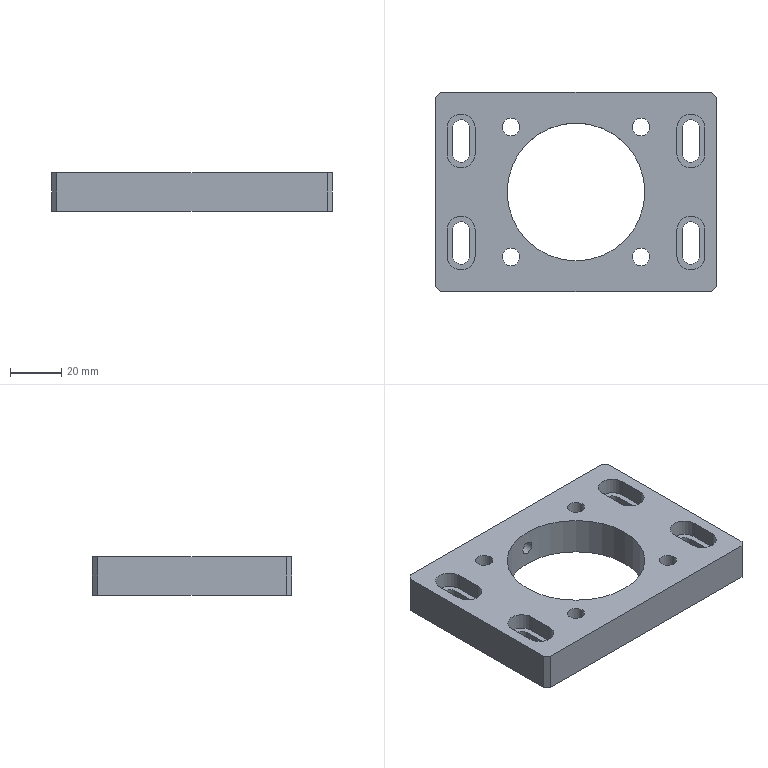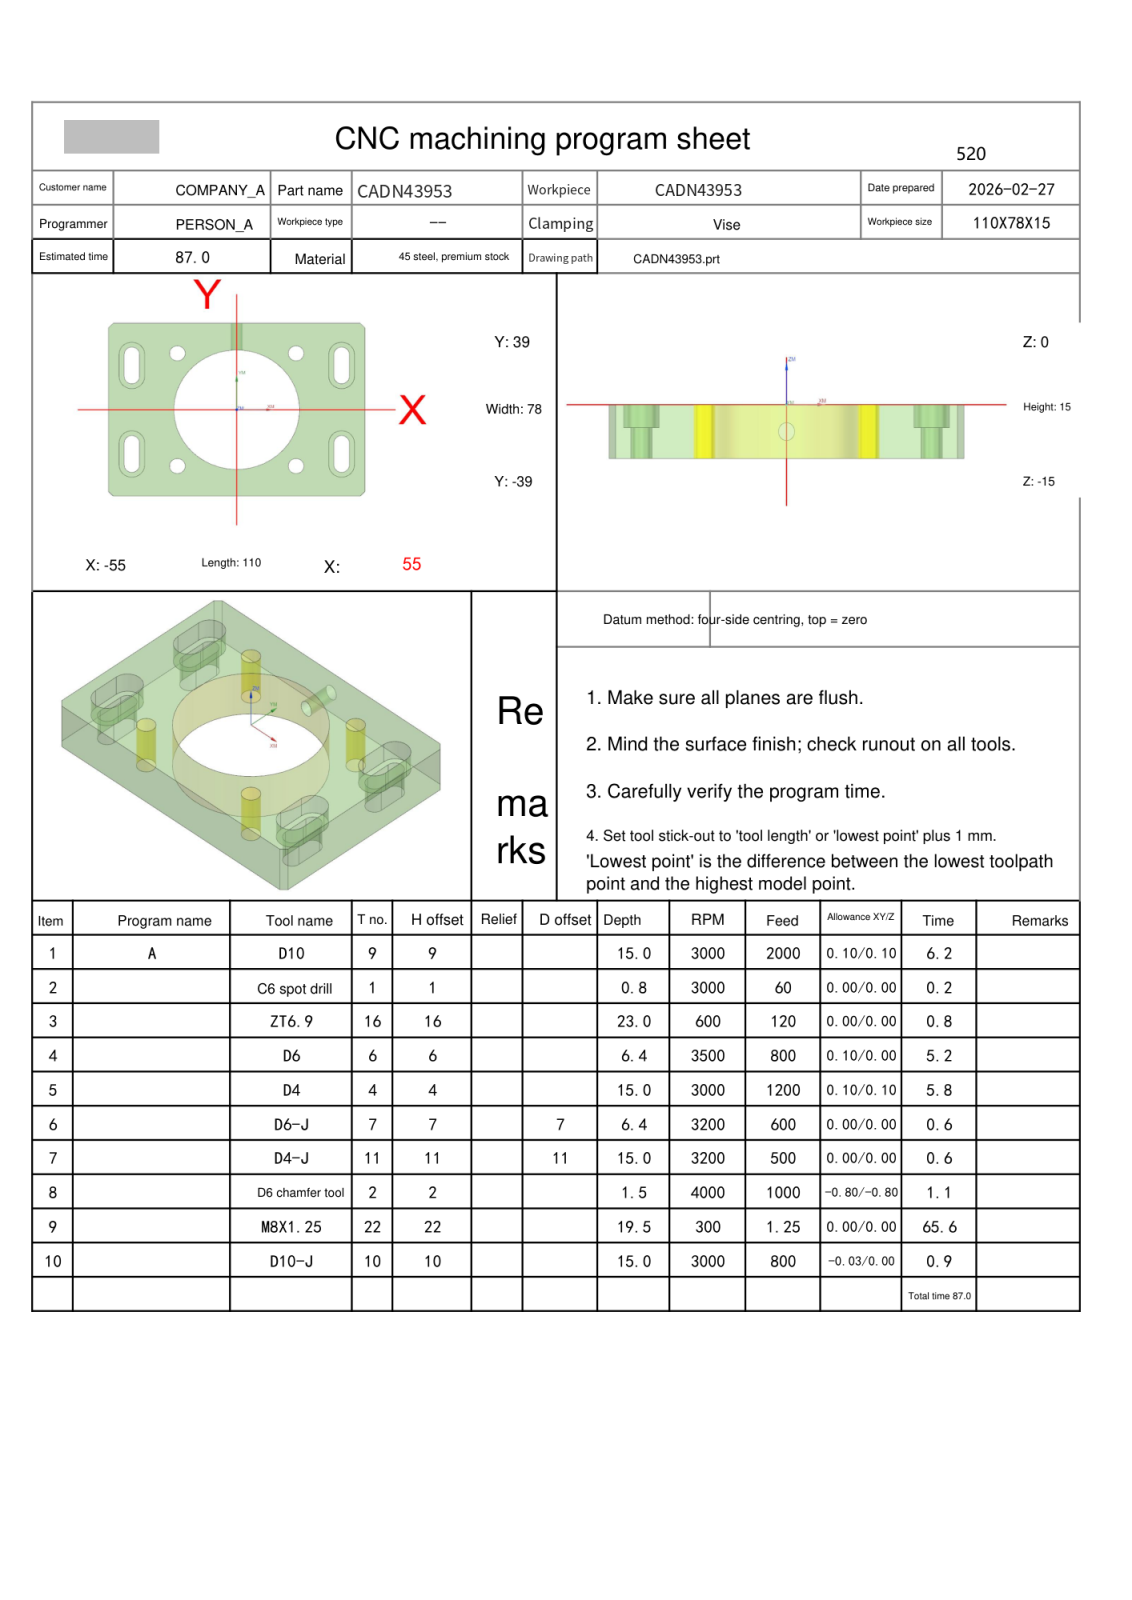NC program | NX | posted by the shop | part box 110 x 78 x 15 mm
Lines 4089 to 4469 of 4469:
N8 T02 M06
(D6 chamfer tool  D=6. R=0. H=02 ce=-0.80 di=0.00)
G00 G90 G54 X-26.256 Y26.956 M03 S4000
G43 H02 Z50.
M08
Z-1.
G01 Z-1.5 F500.
X-26.656
G03 X-28.156 Y25.456 I0.0 J-1.5
X-25.456 Y22.756 I2.7 J0.0
X-22.756 Y25.456 I0.0 J2.7
X-25.456 Y28.156 I-2.7 J0.0
X-28.156 Y25.456 I0.0 J-2.7
X-26.656 Y23.956 I1.5 J0.0
G01 X-26.256
Z-1.
G00 Z50.
X24.656 Y26.956
Z-1.
G01 Z-1.5
X24.256
G03 X22.756 Y25.456 I0.0 J-1.5
X25.456 Y22.756 I2.7 J0.0
X28.156 Y25.456 I0.0 J2.7
X25.456 Y28.156 I-2.7 J0.0
X22.756 Y25.456 I0.0 J-2.7
X24.256 Y23.956 I1.5 J0.0
G01 X24.656
Z-1.
G00 Z50.
Y-23.956
Z-1.
G01 Z-1.5
X24.256
G03 X22.756 Y-25.456 I0.0 J-1.5
X25.456 Y-28.156 I2.7 J0.0
X28.156 Y-25.456 I0.0 J2.7
X25.456 Y-22.756 I-2.7 J0.0
X22.756 Y-25.456 I0.0 J-2.7
X24.256 Y-26.956 I1.5 J0.0
G01 X24.656
Z-1.
G00 Z50.
X-26.256 Y-23.956
Z-1.
G01 Z-1.5
X-26.656
G03 X-28.156 Y-25.456 I0.0 J-1.5
X-25.456 Y-28.156 I2.7 J0.0
X-22.756 Y-25.456 I0.0 J2.7
X-25.456 Y-22.756 I-2.7 J0.0
X-28.156 Y-25.456 I0.0 J-2.7
X-26.656 Y-26.956 I1.5 J0.0
G01 X-26.256
Z-1.
G00 Z50.
G00 G90 X-.386 Y40.227 M03 S3500
Z50.
Z.172
G01 Z-1.2 F1000.
G03 X-.1 Y40.027 I1.286 J1.532
G01 X-.054 Y39.997
X0.0 Y40.
X53.
X53.259 Y39.966
X53.5 Y39.866
X53.707 Y39.707
X55.707 Y37.707
X55.866 Y37.5
X55.966 Y37.259
X56. Y37.
Y-37.
X55.966 Y-37.259
X55.866 Y-37.5
X55.707 Y-37.707
X53.707 Y-39.707
X53.5 Y-39.866
X53.259 Y-39.966
X53. Y-40.
X-53.
X-53.259 Y-39.966
X-53.5 Y-39.866
X-53.707 Y-39.707
X-55.707 Y-37.707
X-55.866 Y-37.5
X-55.966 Y-37.259
X-56. Y-37.
Y37.
X-55.966 Y37.259
X-55.866 Y37.5
X-55.707 Y37.707
X-53.707 Y39.707
X-53.5 Y39.866
X-53.259 Y39.966
X-53. Y40.
X0.0
X.054 Y39.997
X.1 Y40.027
G03 X.386 Y40.227 I-1. J1.732
G01 Z.172
G00 Z10.
X-40.727 Y19.614
Z.172
G01 Z-1.2
G03 X-40.527 Y19.9 I-1.532 J1.286
G01 X-40.497 Y19.946
X-40.5 Y20.
Y25.
G03 X-45. Y29.5 I-4.5 J0.0
X-49.5 Y25. I0.0 J-4.5
G01 Y15.
G03 X-45. Y10.5 I4.5 J0.0
X-40.5 Y15. I0.0 J4.5
G01 Y20.
X-40.497 Y20.054
X-40.527 Y20.1
G03 X-40.727 Y20.386 I-1.732 J-1.
G01 Z.172
G00 Z10.
X-27.664 Y25.86
Z.252
G01 Z-1.2
G03 X-27.838 Y25.558 I1.638 J-1.147
G01 X-27.863 Y25.51
X-27.856 Y25.456
G03 X-25.456 Y23.056 I2.4 J0.0
X-23.056 Y25.456 I0.0 J2.4
X-25.456 Y27.856 I-2.4 J0.0
X-27.856 Y25.456 I0.0 J-2.4
G01 X-27.863 Y25.402
X-27.838 Y25.354
G03 X-27.664 Y25.052 I1.813 J.845
G01 Z.252
G00 Z10.
X-40.727 Y-20.386
Z.172
G01 Z-1.2
G03 X-40.527 Y-20.1 I-1.532 J1.286
G01 X-40.497 Y-20.054
X-40.5 Y-20.
Y-15.
G03 X-45. Y-10.5 I-4.5 J0.0
X-49.5 Y-15. I0.0 J-4.5
G01 Y-25.
G03 X-45. Y-29.5 I4.5 J0.0
X-40.5 Y-25. I0.0 J4.5
G01 Y-20.
X-40.497 Y-19.946
X-40.527 Y-19.9
G03 X-40.727 Y-19.614 I-1.732 J-1.
G01 Z.172
G00 Z10.
X-27.664 Y-25.052
Z.252
G01 Z-1.2
G03 X-27.838 Y-25.354 I1.638 J-1.147
G01 X-27.863 Y-25.402
X-27.856 Y-25.456
G03 X-25.456 Y-27.856 I2.4 J0.0
X-23.056 Y-25.456 I0.0 J2.4
X-25.456 Y-23.056 I-2.4 J0.0
X-27.856 Y-25.456 I0.0 J-2.4
G01 X-27.863 Y-25.51
X-27.838 Y-25.558
G03 X-27.664 Y-25.86 I1.813 J.845
G01 Z.252
G00 Z10.
X-25.784 Y.392
Z.194
G01 Z-1.2
G03 X-25.976 Y.101 I1.567 J-1.243
G01 X-26.004 Y.054
X-26. Y0.0
G03 X0.0 Y-26. I26. J0.0
X26. Y0.0 I0.0 J26.
X0.0 Y26. I-26. J0.0
X-26. Y0.0 I0.0 J-26.
G01 X-26.004 Y-.054
X-25.976 Y-.101
G03 X-25.784 Y-.392 I1.759 J.952
G01 Z.194
G00 Z10.
X23.248 Y-25.052
Z.252
G01 Z-1.2
G03 X23.074 Y-25.354 I1.638 J-1.147
G01 X23.048 Y-25.402
X23.056 Y-25.456
G03 X25.456 Y-27.856 I2.4 J0.0
X27.856 Y-25.456 I0.0 J2.4
X25.456 Y-23.056 I-2.4 J0.0
X23.056 Y-25.456 I0.0 J-2.4
G01 X23.048 Y-25.51
X23.074 Y-25.558
G03 X23.248 Y-25.86 I1.813 J.845
G01 Z.252
G00 Z10.
X40.727 Y-19.614
Z.172
G01 Z-1.2
G03 X40.527 Y-19.9 I1.532 J-1.286
G01 X40.497 Y-19.946
X40.5 Y-20.
Y-25.
G03 X45. Y-29.5 I4.5 J0.0
X49.5 Y-25. I0.0 J4.5
G01 Y-15.
G03 X45. Y-10.5 I-4.5 J0.0
X40.5 Y-15. I0.0 J-4.5
G01 Y-20.
X40.497 Y-20.054
X40.527 Y-20.1
G03 X40.727 Y-20.386 I1.732 J1.
G01 Z.172
G00 Z10.
X49.273 Y19.614
Z.172
G01 Z-1.2
G03 X49.473 Y19.9 I-1.532 J1.286
G01 X49.503 Y19.946
X49.5 Y20.
Y25.
G03 X45. Y29.5 I-4.5 J0.0
X40.5 Y25. I0.0 J-4.5
G01 Y15.
G03 X45. Y10.5 I4.5 J0.0
X49.5 Y15. I0.0 J4.5
G01 Y20.
X49.503 Y20.054
X49.473 Y20.1
G03 X49.273 Y20.386 I-1.732 J-1.
G01 Z.172
G00 Z10.
X23.248 Y25.86
Z.252
G01 Z-1.2
G03 X23.074 Y25.558 I1.638 J-1.147
G01 X23.048 Y25.51
X23.056 Y25.456
G03 X25.456 Y23.056 I2.4 J0.0
X27.856 Y25.456 I0.0 J2.4
X25.456 Y27.856 I-2.4 J0.0
X23.056 Y25.456 I0.0 J-2.4
G01 X23.048 Y25.402
X23.074 Y25.354
G03 X23.248 Y25.052 I1.813 J.845
G01 Z.252
G00 Z50.
G91 G28 Z0.0
M05
M09
G91 G28 Z0.0
M01
N9 T22 M06
(M8X1.25 D=6.8 DR_a=180 H=22)
G00 G90 G54 X25.456 Y25.456 M03 S300
G43 H22 Z50.
M08
G95
G98 G84 X25.456 Y25.456 Z-19.5 R1. F1.25 Q3.
Y-25.456
X-25.456
Y25.456
G80
G94
G00 Z50.
G91 G28 Z0.0
M05
M09
G91 G28 Z0.0
M01
N10 T10 M06
(D10-J  D=10. R=0. H=10 ce=0.00 di=0.00)
G00 G90 G54 X52.293 Y46.778 M03 S3000
G43 H10 Z50.
M08
Z-7.
G01 Z-8. F800.
X56.536 Y42.536
X58.536 Y40.536
X62.778 Y36.293
Z-7.
G00 Z50.
Y-36.293
Z-7.
G01 Z-8.
X58.536 Y-40.536
X56.536 Y-42.536
X52.293 Y-46.778
Z-7.
G00 Z50.
X-52.293
Z-7.
G01 Z-8.
X-56.536 Y-42.536
X-58.536 Y-40.536
X-62.778 Y-36.293
Z-7.
G00 Z50.
Y36.293
Z-7.
G01 Z-8.
X-58.536 Y40.536
X-56.536 Y42.536
X-52.293 Y46.778
Z-7.
G00 Z50.
G00 G90 X-1.5 Y-20.27 M03 S3000
Z10.
Z-6.
G01 Z-7.5 F800.
G41 D10
Y-20.525
G03 X0.0 Y-22.025 I1.5 J0.0
X22.025 Y0.0 I0.0 J22.025
X0.0 Y22.025 I-22.025 J0.0
X-22.025 Y0.0 I0.0 J-22.025
X0.0 Y-22.025 I22.025 J0.0
X.4 Y-22.021 I0.0 J22.025
X1.873 Y-20.522 I-.027 J1.5
G01 X1.872 Y-20.494
X1.871 Y-20.44
G40 X1.868 Y-20.24
Z-6.
G00 X-1.5 Y-20.27
Z-13.5
G01 Z-15.
G41 D10
Y-20.525
G03 X0.0 Y-22.025 I1.5 J0.0
X22.025 Y0.0 I0.0 J22.025
X0.0 Y22.025 I-22.025 J0.0
X-22.025 Y0.0 I0.0 J-22.025
X0.0 Y-22.025 I22.025 J0.0
X.4 Y-22.021 I0.0 J22.025
X1.873 Y-20.522 I-.027 J1.5
G01 X1.872 Y-20.494
X1.871 Y-20.44
G40 X1.868 Y-20.24
Z-13.5
G00 Z10.
G00 G90 X-1.5 Y-20.27 M03 S3000
Z10.
Z-6.
G01 Z-7.5 F800.
G41 D10
Y-20.525
G03 X0.0 Y-22.025 I1.5 J0.0
X22.025 Y0.0 I0.0 J22.025
X0.0 Y22.025 I-22.025 J0.0
X-22.025 Y0.0 I0.0 J-22.025
X0.0 Y-22.025 I22.025 J0.0
X.4 Y-22.021 I0.0 J22.025
X1.873 Y-20.522 I-.027 J1.5
G01 X1.872 Y-20.494
X1.871 Y-20.44
G40 X1.868 Y-20.24
Z-6.
G00 X-1.5 Y-20.27
Z-13.5
G01 Z-15.
G41 D10
Y-20.525
G03 X0.0 Y-22.025 I1.5 J0.0
X22.025 Y0.0 I0.0 J22.025
X0.0 Y22.025 I-22.025 J0.0
X-22.025 Y0.0 I0.0 J-22.025
X0.0 Y-22.025 I22.025 J0.0
X.4 Y-22.021 I0.0 J22.025
X1.873 Y-20.522 I-.027 J1.5
G01 X1.872 Y-20.494
X1.871 Y-20.44
G40 X1.868 Y-20.24
Z-13.5
G00 Z10.
M05
M09
G91 G28 Z0.0
G91 G28 Y0.0
M30
%